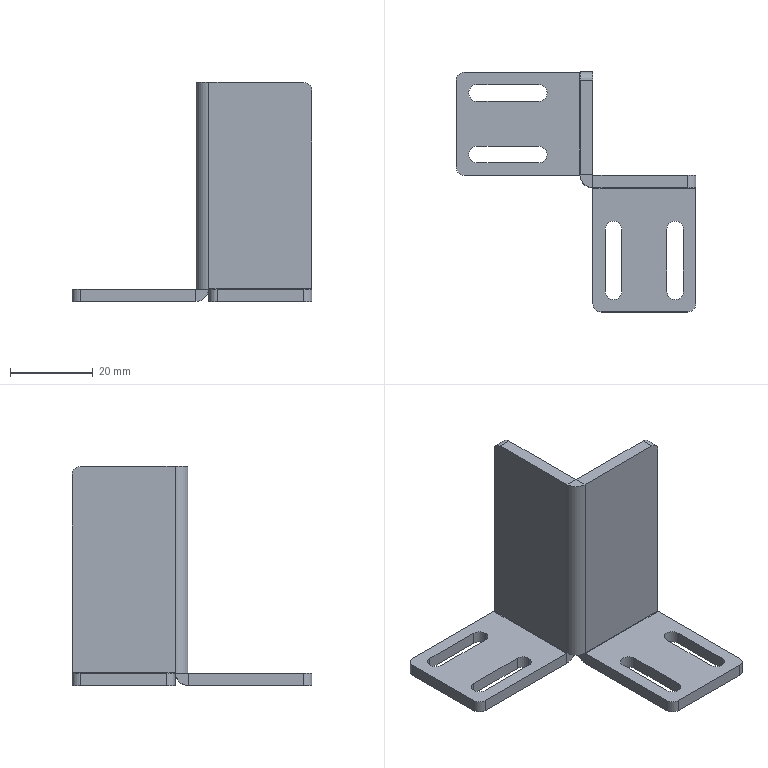Part | STEP file | PClimit part | 1 solid | 54 faces | box 58 x 58 x 53 mm | volume 11788 mm3 | plane 32 | cylinder 22 | commonest cylinder face diameters 4 x16 0.2 x3 6.2 x3